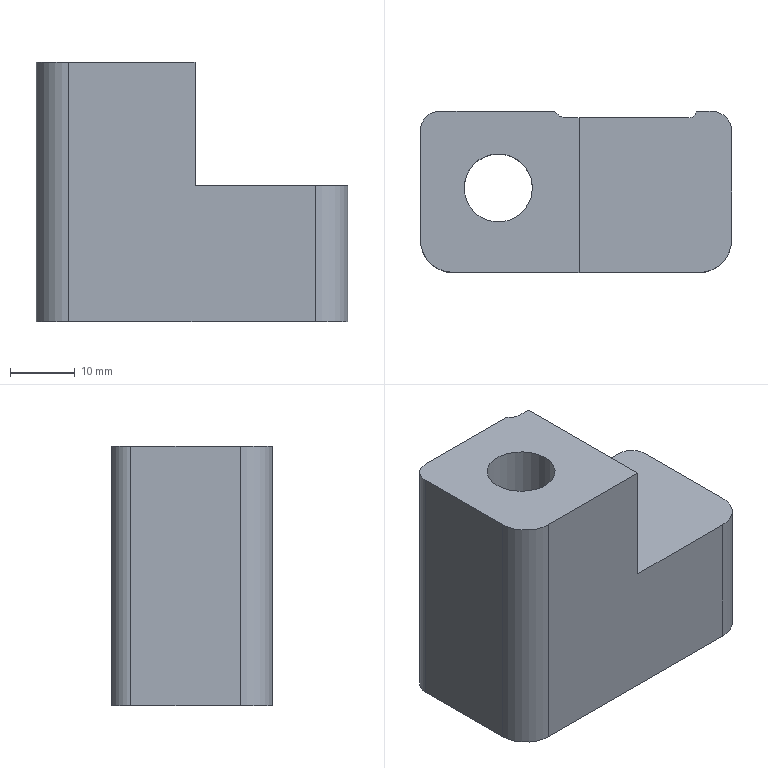Part | NX | features PS-11 2 | 1 solid | 19 faces | box 47.924 x 24.8 x 40 mm | volume 29874 mm3 | plane 11 | cylinder 8 | commonest cylinder face diameters 6 x2 10 x2 2.4 x1 4.4 x1 10.5 x1 18 x1
STEP:
#1=CARTESIAN_POINT('',(2543.009,-914.397,881.716));
#2=VERTEX_POINT('',#1);
#3=CARTESIAN_POINT('',(2543.009,-938.197,881.716));
#4=VERTEX_POINT('',#3);
#5=CARTESIAN_POINT('',(2543.009,-857.123,881.716));
#6=DIRECTION('',(0.,-1.,0.));
#7=VECTOR('',#6,1000.);
#8=LINE('',#5,#7);
#9=EDGE_CURVE('',#2,#4,#8,.T.);
#10=ORIENTED_EDGE('',*,*,#9,.F.);
#11=CARTESIAN_POINT('',(2543.009,-914.397,900.716));
#12=VERTEX_POINT('',#11);
#13=CARTESIAN_POINT('',(2543.009,-914.397,940.716));
#14=DIRECTION('',(0.,0.,-1.));
#15=VECTOR('',#14,1000.);
#16=LINE('',#13,#15);
#17=EDGE_CURVE('',#12,#2,#16,.T.);
#18=ORIENTED_EDGE('',*,*,#17,.F.);
#19=CARTESIAN_POINT('',(2543.009,-938.197,900.716));
#20=VERTEX_POINT('',#19);
#21=CARTESIAN_POINT('',(2543.009,-857.123,900.716));
#22=DIRECTION('',(0.,-1.,0.));
#23=VECTOR('',#22,1000.);
#24=LINE('',#21,#23);
#25=EDGE_CURVE('',#20,#12,#24,.F.);
#26=ORIENTED_EDGE('',*,*,#25,.F.);
#27=CARTESIAN_POINT('',(2543.009,-938.197,853.217));
#28=DIRECTION('',(0.,0.,-1.));
#29=VECTOR('',#28,1000.);
#30=LINE('',#27,#29);
#31=EDGE_CURVE('',#4,#20,#30,.F.);
#32=ORIENTED_EDGE('',*,*,#31,.F.);
#33=EDGE_LOOP('',(#10,#18,#26,#32));
#34=FACE_BOUND('',#33,.T.);
#35=CARTESIAN_POINT('',(2543.009,-923.947,911.056));
#36=DIRECTION('',(-1.,0.,0.));
#37=DIRECTION('',(0.,0.,1.));
#38=AXIS2_PLACEMENT_3D('',#35,#36,#37);
#39=PLANE('',#38);
#40=ADVANCED_FACE('',(#34),#39,.F.);
#41=CARTESIAN_POINT('',(2559.923,-914.397,860.716));
#42=VERTEX_POINT('',#41);
#43=CARTESIAN_POINT('',(2541.096,-914.397,860.716));
#44=VERTEX_POINT('',#43);
#45=CARTESIAN_POINT('',(2585.094,-914.397,860.716));
#46=DIRECTION('',(-1.,0.,0.));
#47=VECTOR('',#46,1000.);
#48=LINE('',#45,#47);
#49=EDGE_CURVE('',#42,#44,#48,.T.);
#50=ORIENTED_EDGE('',*,*,#49,.F.);
#51=CARTESIAN_POINT('',(2561.106,-913.397,860.716));
#52=VERTEX_POINT('',#51);
#53=CARTESIAN_POINT('',(2559.923,-913.197,860.716));
#54=DIRECTION('',(0.,0.,-1.));
#55=DIRECTION('',(-1.,0.,0.));
#56=AXIS2_PLACEMENT_3D('',#53,#54,#55);
#57=CIRCLE('',#56,1.2);
#58=EDGE_CURVE('',#52,#42,#57,.T.);
#59=ORIENTED_EDGE('',*,*,#58,.F.);
#60=CARTESIAN_POINT('',(2563.509,-913.397,860.716));
#61=VERTEX_POINT('',#60);
#62=CARTESIAN_POINT('',(2585.094,-913.397,860.716));
#63=DIRECTION('',(1.,0.,0.));
#64=VECTOR('',#63,1000.);
#65=LINE('',#62,#64);
#66=EDGE_CURVE('',#52,#61,#65,.T.);
#67=ORIENTED_EDGE('',*,*,#66,.T.);
#68=CARTESIAN_POINT('',(2566.509,-916.397,860.716));
#69=VERTEX_POINT('',#68);
#70=CARTESIAN_POINT('',(2563.509,-916.397,860.716));
#71=DIRECTION('',(0.,0.,-1.));
#72=DIRECTION('',(-1.,0.,0.));
#73=AXIS2_PLACEMENT_3D('',#70,#71,#72);
#74=CIRCLE('',#73,3.);
#75=EDGE_CURVE('',#61,#69,#74,.T.);
#76=ORIENTED_EDGE('',*,*,#75,.T.);
#77=CARTESIAN_POINT('',(2566.509,-933.197,860.716));
#78=VERTEX_POINT('',#77);
#79=CARTESIAN_POINT('',(2566.509,-906.16,860.716));
#80=DIRECTION('',(0.,1.,0.));
#81=VECTOR('',#80,1000.);
#82=LINE('',#79,#81);
#83=EDGE_CURVE('',#78,#69,#82,.T.);
#84=ORIENTED_EDGE('',*,*,#83,.F.);
#85=CARTESIAN_POINT('',(2561.509,-938.197,860.716));
#86=VERTEX_POINT('',#85);
#87=CARTESIAN_POINT('',(2561.509,-933.197,860.716));
#88=DIRECTION('',(0.,0.,1.));
#89=DIRECTION('',(-1.,0.,0.));
#90=AXIS2_PLACEMENT_3D('',#87,#88,#89);
#91=CIRCLE('',#90,5.);
#92=EDGE_CURVE('',#86,#78,#91,.T.);
#93=ORIENTED_EDGE('',*,*,#92,.F.);
#94=CARTESIAN_POINT('',(2523.585,-938.197,860.716));
#95=VERTEX_POINT('',#94);
#96=CARTESIAN_POINT('',(2524.047,-938.197,860.716));
#97=DIRECTION('',(-1.,0.,0.));
#98=VECTOR('',#97,1000.);
#99=LINE('',#96,#98);
#100=EDGE_CURVE('',#86,#95,#99,.T.);
#101=ORIENTED_EDGE('',*,*,#100,.T.);
#102=CARTESIAN_POINT('',(2518.585,-933.197,860.716));
#103=VERTEX_POINT('',#102);
#104=CARTESIAN_POINT('',(2523.585,-933.197,860.716));
#105=DIRECTION('',(0.,0.,1.));
#106=DIRECTION('',(-1.,0.,0.));
#107=AXIS2_PLACEMENT_3D('',#104,#105,#106);
#108=CIRCLE('',#107,5.);
#109=EDGE_CURVE('',#103,#95,#108,.T.);
#110=ORIENTED_EDGE('',*,*,#109,.F.);
#111=CARTESIAN_POINT('',(2518.585,-916.397,860.716));
#112=VERTEX_POINT('',#111);
#113=CARTESIAN_POINT('',(2518.585,-924.697,860.716));
#114=DIRECTION('',(0.,1.,0.));
#115=VECTOR('',#114,1000.);
#116=LINE('',#113,#115);
#117=EDGE_CURVE('',#103,#112,#116,.T.);
#118=ORIENTED_EDGE('',*,*,#117,.T.);
#119=CARTESIAN_POINT('',(2521.585,-913.397,860.716));
#120=VERTEX_POINT('',#119);
#121=CARTESIAN_POINT('',(2521.585,-916.397,860.716));
#122=DIRECTION('',(0.,0.,-1.));
#123=DIRECTION('',(-1.,0.,0.));
#124=AXIS2_PLACEMENT_3D('',#121,#122,#123);
#125=CIRCLE('',#124,3.);
#126=EDGE_CURVE('',#112,#120,#125,.T.);
#127=ORIENTED_EDGE('',*,*,#126,.T.);
#128=CARTESIAN_POINT('',(2539.252,-913.397,860.716));
#129=VERTEX_POINT('',#128);
#130=CARTESIAN_POINT('',(2585.094,-913.397,860.716));
#131=DIRECTION('',(1.,0.,0.));
#132=VECTOR('',#131,1000.);
#133=LINE('',#130,#132);
#134=EDGE_CURVE('',#120,#129,#133,.T.);
#135=ORIENTED_EDGE('',*,*,#134,.T.);
#136=CARTESIAN_POINT('',(2541.096,-912.197,860.716));
#137=DIRECTION('',(0.,0.,-1.));
#138=DIRECTION('',(-1.,0.,0.));
#139=AXIS2_PLACEMENT_3D('',#136,#137,#138);
#140=CIRCLE('',#139,2.2);
#141=EDGE_CURVE('',#129,#44,#140,.F.);
#142=ORIENTED_EDGE('',*,*,#141,.T.);
#143=EDGE_LOOP('',(#50,#59,#67,#76,#84,#93,#101,#110,#118,#127,#135,#142));
#144=FACE_BOUND('',#143,.T.);
#145=CARTESIAN_POINT('',(2521.585,-925.197,860.716));
#146=VERTEX_POINT('',#145);
#147=CARTESIAN_POINT('',(2530.585,-925.197,860.716));
#148=DIRECTION('',(0.,0.,1.));
#149=DIRECTION('',(-1.,0.,0.));
#150=AXIS2_PLACEMENT_3D('',#147,#148,#149);
#151=CIRCLE('',#150,9.);
#152=EDGE_CURVE('',#146,#146,#151,.T.);
#153=ORIENTED_EDGE('',*,*,#152,.T.);
#154=EDGE_LOOP('',(#153));
#155=FACE_BOUND('',#154,.T.);
#156=CARTESIAN_POINT('',(2585.094,-857.123,860.716));
#157=DIRECTION('',(0.,0.,-1.));
#158=DIRECTION('',(-1.,0.,0.));
#159=AXIS2_PLACEMENT_3D('',#156,#157,#158);
#160=PLANE('',#159);
#161=ADVANCED_FACE('',(#144,#155),#160,.T.);
#162=ORIENTED_EDGE('',*,*,#25,.T.);
#163=CARTESIAN_POINT('',(2541.096,-914.397,900.716));
#164=VERTEX_POINT('',#163);
#165=CARTESIAN_POINT('',(2585.094,-914.397,900.716));
#166=DIRECTION('',(1.,0.,0.));
#167=VECTOR('',#166,1000.);
#168=LINE('',#165,#167);
#169=EDGE_CURVE('',#164,#12,#168,.T.);
#170=ORIENTED_EDGE('',*,*,#169,.F.);
#171=CARTESIAN_POINT('',(2539.252,-913.397,900.716));
#172=VERTEX_POINT('',#171);
#173=CARTESIAN_POINT('',(2541.096,-912.197,900.716));
#174=DIRECTION('',(0.,0.,1.));
#175=DIRECTION('',(1.,0.,0.));
#176=AXIS2_PLACEMENT_3D('',#173,#174,#175);
#177=CIRCLE('',#176,2.2);
#178=EDGE_CURVE('',#164,#172,#177,.F.);
#179=ORIENTED_EDGE('',*,*,#178,.T.);
#180=CARTESIAN_POINT('',(2521.585,-913.397,900.716));
#181=VERTEX_POINT('',#180);
#182=CARTESIAN_POINT('',(2585.094,-913.397,900.716));
#183=DIRECTION('',(-1.,0.,0.));
#184=VECTOR('',#183,1000.);
#185=LINE('',#182,#184);
#186=EDGE_CURVE('',#172,#181,#185,.T.);
#187=ORIENTED_EDGE('',*,*,#186,.T.);
#188=CARTESIAN_POINT('',(2518.585,-916.397,900.716));
#189=VERTEX_POINT('',#188);
#190=CARTESIAN_POINT('',(2521.585,-916.397,900.716));
#191=DIRECTION('',(0.,0.,1.));
#192=DIRECTION('',(1.,0.,0.));
#193=AXIS2_PLACEMENT_3D('',#190,#191,#192);
#194=CIRCLE('',#193,3.);
#195=EDGE_CURVE('',#181,#189,#194,.T.);
#196=ORIENTED_EDGE('',*,*,#195,.T.);
#197=CARTESIAN_POINT('',(2518.585,-933.197,900.716));
#198=VERTEX_POINT('',#197);
#199=CARTESIAN_POINT('',(2518.585,-924.697,900.716));
#200=DIRECTION('',(0.,1.,0.));
#201=VECTOR('',#200,1000.);
#202=LINE('',#199,#201);
#203=EDGE_CURVE('',#198,#189,#202,.T.);
#204=ORIENTED_EDGE('',*,*,#203,.F.);
#205=CARTESIAN_POINT('',(2523.585,-938.197,900.716));
#206=VERTEX_POINT('',#205);
#207=CARTESIAN_POINT('',(2523.585,-933.197,900.716));
#208=DIRECTION('',(0.,0.,1.));
#209=DIRECTION('',(1.,0.,0.));
#210=AXIS2_PLACEMENT_3D('',#207,#208,#209);
#211=CIRCLE('',#210,5.);
#212=EDGE_CURVE('',#206,#198,#211,.F.);
#213=ORIENTED_EDGE('',*,*,#212,.F.);
#214=CARTESIAN_POINT('',(2524.047,-938.197,900.716));
#215=DIRECTION('',(-1.,0.,0.));
#216=VECTOR('',#215,1000.);
#217=LINE('',#214,#216);
#218=EDGE_CURVE('',#20,#206,#217,.T.);
#219=ORIENTED_EDGE('',*,*,#218,.F.);
#220=EDGE_LOOP('',(#162,#170,#179,#187,#196,#204,#213,#219));
#221=FACE_BOUND('',#220,.T.);
#222=CARTESIAN_POINT('',(2535.835,-925.197,900.716));
#223=VERTEX_POINT('',#222);
#224=CARTESIAN_POINT('',(2530.585,-925.197,900.716));
#225=DIRECTION('',(0.,0.,1.));
#226=DIRECTION('',(1.,0.,0.));
#227=AXIS2_PLACEMENT_3D('',#224,#225,#226);
#228=CIRCLE('',#227,5.25);
#229=EDGE_CURVE('',#223,#223,#228,.F.);
#230=ORIENTED_EDGE('',*,*,#229,.T.);
#231=EDGE_LOOP('',(#230));
#232=FACE_BOUND('',#231,.T.);
#233=CARTESIAN_POINT('',(2585.094,-857.123,900.716));
#234=DIRECTION('',(0.,0.,1.));
#235=DIRECTION('',(1.,0.,0.));
#236=AXIS2_PLACEMENT_3D('',#233,#234,#235);
#237=PLANE('',#236);
#238=ADVANCED_FACE('',(#221,#232),#237,.T.);
#239=ORIENTED_EDGE('',*,*,#141,.F.);
#240=CARTESIAN_POINT('',(2539.252,-913.397,889.83));
#241=DIRECTION('',(0.,0.,-1.));
#242=VECTOR('',#241,1000.);
#243=LINE('',#240,#242);
#244=EDGE_CURVE('',#129,#172,#243,.F.);
#245=ORIENTED_EDGE('',*,*,#244,.T.);
#246=ORIENTED_EDGE('',*,*,#178,.F.);
#247=CARTESIAN_POINT('',(2541.096,-914.397,940.716));
#248=DIRECTION('',(0.,0.,-1.));
#249=VECTOR('',#248,1000.);
#250=LINE('',#247,#249);
#251=EDGE_CURVE('',#44,#164,#250,.F.);
#252=ORIENTED_EDGE('',*,*,#251,.F.);
#253=EDGE_LOOP('',(#239,#245,#246,#252));
#254=FACE_BOUND('',#253,.T.);
#255=CARTESIAN_POINT('',(2541.096,-912.197,889.83));
#256=DIRECTION('',(0.,0.,-1.));
#257=DIRECTION('',(-1.,0.,0.));
#258=AXIS2_PLACEMENT_3D('',#255,#256,#257);
#259=CYLINDRICAL_SURFACE('',#258,2.2);
#260=ADVANCED_FACE('',(#254),#259,.F.);
#261=ORIENTED_EDGE('',*,*,#100,.F.);
#262=CARTESIAN_POINT('',(2561.509,-938.197,881.716));
#263=VERTEX_POINT('',#262);
#264=CARTESIAN_POINT('',(2561.509,-938.197,853.217));
#265=DIRECTION('',(0.,0.,1.));
#266=VECTOR('',#265,1000.);
#267=LINE('',#264,#266);
#268=EDGE_CURVE('',#263,#86,#267,.F.);
#269=ORIENTED_EDGE('',*,*,#268,.F.);
#270=CARTESIAN_POINT('',(2524.047,-938.197,881.716));
#271=DIRECTION('',(-1.,0.,0.));
#272=VECTOR('',#271,1000.);
#273=LINE('',#270,#272);
#274=EDGE_CURVE('',#263,#4,#273,.T.);
#275=ORIENTED_EDGE('',*,*,#274,.T.);
#276=ORIENTED_EDGE('',*,*,#31,.T.);
#277=ORIENTED_EDGE('',*,*,#218,.T.);
#278=CARTESIAN_POINT('',(2523.585,-938.197,853.217));
#279=DIRECTION('',(0.,0.,1.));
#280=VECTOR('',#279,1000.);
#281=LINE('',#278,#280);
#282=EDGE_CURVE('',#95,#206,#281,.T.);
#283=ORIENTED_EDGE('',*,*,#282,.F.);
#284=EDGE_LOOP('',(#261,#269,#275,#276,#277,#283));
#285=FACE_BOUND('',#284,.T.);
#286=CARTESIAN_POINT('',(2524.047,-938.197,853.217));
#287=DIRECTION('',(0.,-1.,0.));
#288=DIRECTION('',(0.,0.,1.));
#289=AXIS2_PLACEMENT_3D('',#286,#287,#288);
#290=PLANE('',#289);
#291=ADVANCED_FACE('',(#285),#290,.T.);
#292=ORIENTED_EDGE('',*,*,#203,.T.);
#293=CARTESIAN_POINT('',(2518.585,-916.397,875.716));
#294=DIRECTION('',(0.,0.,-1.));
#295=VECTOR('',#294,1000.);
#296=LINE('',#293,#295);
#297=EDGE_CURVE('',#189,#112,#296,.T.);
#298=ORIENTED_EDGE('',*,*,#297,.T.);
#299=ORIENTED_EDGE('',*,*,#117,.F.);
#300=CARTESIAN_POINT('',(2518.585,-933.197,875.716));
#301=DIRECTION('',(0.,0.,1.));
#302=VECTOR('',#301,1000.);
#303=LINE('',#300,#302);
#304=EDGE_CURVE('',#198,#103,#303,.F.);
#305=ORIENTED_EDGE('',*,*,#304,.F.);
#306=EDGE_LOOP('',(#292,#298,#299,#305));
#307=FACE_BOUND('',#306,.T.);
#308=CARTESIAN_POINT('',(2518.585,-924.697,875.716));
#309=DIRECTION('',(-1.,0.,0.));
#310=DIRECTION('',(0.,0.,1.));
#311=AXIS2_PLACEMENT_3D('',#308,#309,#310);
#312=PLANE('',#311);
#313=ADVANCED_FACE('',(#307),#312,.T.);
#314=ORIENTED_EDGE('',*,*,#109,.T.);
#315=ORIENTED_EDGE('',*,*,#282,.T.);
#316=ORIENTED_EDGE('',*,*,#212,.T.);
#317=ORIENTED_EDGE('',*,*,#304,.T.);
#318=EDGE_LOOP('',(#314,#315,#316,#317));
#319=FACE_BOUND('',#318,.T.);
#320=CARTESIAN_POINT('',(2523.585,-933.197,853.217));
#321=DIRECTION('',(0.,0.,1.));
#322=DIRECTION('',(1.,0.,0.));
#323=AXIS2_PLACEMENT_3D('',#320,#321,#322);
#324=CYLINDRICAL_SURFACE('',#323,5.);
#325=ADVANCED_FACE('',(#319),#324,.T.);
#326=ORIENTED_EDGE('',*,*,#229,.F.);
#327=EDGE_LOOP('',(#326));
#328=FACE_BOUND('',#327,.T.);
#329=CARTESIAN_POINT('',(2525.335,-925.197,873.716));
#330=VERTEX_POINT('',#329);
#331=CARTESIAN_POINT('',(2530.585,-925.197,873.716));
#332=DIRECTION('',(0.,0.,1.));
#333=DIRECTION('',(-1.,0.,0.));
#334=AXIS2_PLACEMENT_3D('',#331,#332,#333);
#335=CIRCLE('',#334,5.25);
#336=EDGE_CURVE('',#330,#330,#335,.T.);
#337=ORIENTED_EDGE('',*,*,#336,.F.);
#338=EDGE_LOOP('',(#337));
#339=FACE_BOUND('',#338,.T.);
#340=CARTESIAN_POINT('',(2530.585,-925.197,891.716));
#341=DIRECTION('',(0.,0.,-1.));
#342=DIRECTION('',(-1.,0.,0.));
#343=AXIS2_PLACEMENT_3D('',#340,#341,#342);
#344=CYLINDRICAL_SURFACE('',#343,5.25);
#345=ADVANCED_FACE('',(#328,#339),#344,.F.);
#346=ORIENTED_EDGE('',*,*,#152,.F.);
#347=EDGE_LOOP('',(#346));
#348=FACE_BOUND('',#347,.T.);
#349=CARTESIAN_POINT('',(2539.585,-925.197,873.716));
#350=VERTEX_POINT('',#349);
#351=CARTESIAN_POINT('',(2530.585,-925.197,873.716));
#352=DIRECTION('',(0.,0.,1.));
#353=DIRECTION('',(1.,0.,0.));
#354=AXIS2_PLACEMENT_3D('',#351,#352,#353);
#355=CIRCLE('',#354,9.);
#356=EDGE_CURVE('',#350,#350,#355,.F.);
#357=ORIENTED_EDGE('',*,*,#356,.F.);
#358=EDGE_LOOP('',(#357));
#359=FACE_BOUND('',#358,.T.);
#360=CARTESIAN_POINT('',(2530.585,-925.197,873.716));
#361=DIRECTION('',(0.,0.,-1.));
#362=DIRECTION('',(-1.,0.,0.));
#363=AXIS2_PLACEMENT_3D('',#360,#361,#362);
#364=CYLINDRICAL_SURFACE('',#363,9.);
#365=ADVANCED_FACE('',(#348,#359),#364,.F.);
#366=ORIENTED_EDGE('',*,*,#336,.T.);
#367=EDGE_LOOP('',(#366));
#368=FACE_BOUND('',#367,.T.);
#369=ORIENTED_EDGE('',*,*,#356,.T.);
#370=EDGE_LOOP('',(#369));
#371=FACE_BOUND('',#370,.T.);
#372=CARTESIAN_POINT('',(2530.585,-925.197,873.716));
#373=DIRECTION('',(0.,0.,-1.));
#374=DIRECTION('',(-1.,0.,0.));
#375=AXIS2_PLACEMENT_3D('',#372,#373,#374);
#376=PLANE('',#375);
#377=ADVANCED_FACE('',(#368,#371),#376,.T.);
#378=ORIENTED_EDGE('',*,*,#169,.T.);
#379=ORIENTED_EDGE('',*,*,#17,.T.);
#380=CARTESIAN_POINT('',(2559.923,-914.397,881.716));
#381=VERTEX_POINT('',#380);
#382=CARTESIAN_POINT('',(2585.094,-914.397,881.716));
#383=DIRECTION('',(1.,0.,0.));
#384=VECTOR('',#383,1000.);
#385=LINE('',#382,#384);
#386=EDGE_CURVE('',#2,#381,#385,.T.);
#387=ORIENTED_EDGE('',*,*,#386,.T.);
#388=CARTESIAN_POINT('',(2559.923,-914.397,940.716));
#389=DIRECTION('',(0.,0.,-1.));
#390=VECTOR('',#389,1000.);
#391=LINE('',#388,#390);
#392=EDGE_CURVE('',#42,#381,#391,.F.);
#393=ORIENTED_EDGE('',*,*,#392,.F.);
#394=ORIENTED_EDGE('',*,*,#49,.T.);
#395=ORIENTED_EDGE('',*,*,#251,.T.);
#396=EDGE_LOOP('',(#378,#379,#387,#393,#394,#395));
#397=FACE_BOUND('',#396,.T.);
#398=CARTESIAN_POINT('',(2656.665,-914.397,940.716));
#399=DIRECTION('',(0.,-1.,0.));
#400=DIRECTION('',(0.,0.,-1.));
#401=AXIS2_PLACEMENT_3D('',#398,#399,#400);
#402=PLANE('',#401);
#403=ADVANCED_FACE('',(#397),#402,.F.);
#404=ORIENTED_EDGE('',*,*,#134,.F.);
#405=CARTESIAN_POINT('',(2521.585,-913.397,875.716));
#406=DIRECTION('',(0.,0.,-1.));
#407=VECTOR('',#406,1000.);
#408=LINE('',#405,#407);
#409=EDGE_CURVE('',#120,#181,#408,.F.);
#410=ORIENTED_EDGE('',*,*,#409,.T.);
#411=ORIENTED_EDGE('',*,*,#186,.F.);
#412=ORIENTED_EDGE('',*,*,#244,.F.);
#413=EDGE_LOOP('',(#404,#410,#411,#412));
#414=FACE_BOUND('',#413,.T.);
#415=CARTESIAN_POINT('',(2550.509,-913.397,875.716));
#416=DIRECTION('',(0.,1.,0.));
#417=DIRECTION('',(0.,0.,1.));
#418=AXIS2_PLACEMENT_3D('',#415,#416,#417);
#419=PLANE('',#418);
#420=ADVANCED_FACE('',(#414),#419,.T.);
#421=ORIENTED_EDGE('',*,*,#195,.F.);
#422=ORIENTED_EDGE('',*,*,#409,.F.);
#423=ORIENTED_EDGE('',*,*,#126,.F.);
#424=ORIENTED_EDGE('',*,*,#297,.F.);
#425=EDGE_LOOP('',(#421,#422,#423,#424));
#426=FACE_BOUND('',#425,.T.);
#427=CARTESIAN_POINT('',(2521.585,-916.397,875.716));
#428=DIRECTION('',(0.,0.,-1.));
#429=DIRECTION('',(-1.,0.,0.));
#430=AXIS2_PLACEMENT_3D('',#427,#428,#429);
#431=CYLINDRICAL_SURFACE('',#430,3.);
#432=ADVANCED_FACE('',(#426),#431,.T.);
#433=CARTESIAN_POINT('',(2563.509,-913.397,881.716));
#434=VERTEX_POINT('',#433);
#435=CARTESIAN_POINT('',(2561.106,-913.397,881.716));
#436=VERTEX_POINT('',#435);
#437=CARTESIAN_POINT('',(2585.094,-913.397,881.716));
#438=DIRECTION('',(-1.,0.,0.));
#439=VECTOR('',#438,1000.);
#440=LINE('',#437,#439);
#441=EDGE_CURVE('',#434,#436,#440,.T.);
#442=ORIENTED_EDGE('',*,*,#441,.F.);
#443=CARTESIAN_POINT('',(2563.509,-913.397,875.716));
#444=DIRECTION('',(0.,0.,1.));
#445=VECTOR('',#444,1000.);
#446=LINE('',#443,#445);
#447=EDGE_CURVE('',#434,#61,#446,.F.);
#448=ORIENTED_EDGE('',*,*,#447,.T.);
#449=ORIENTED_EDGE('',*,*,#66,.F.);
#450=CARTESIAN_POINT('',(2561.106,-913.397,940.716));
#451=DIRECTION('',(0.,0.,-1.));
#452=VECTOR('',#451,1000.);
#453=LINE('',#450,#452);
#454=EDGE_CURVE('',#52,#436,#453,.F.);
#455=ORIENTED_EDGE('',*,*,#454,.T.);
#456=EDGE_LOOP('',(#442,#448,#449,#455));
#457=FACE_BOUND('',#456,.T.);
#458=CARTESIAN_POINT('',(2550.509,-913.397,875.716));
#459=DIRECTION('',(0.,1.,0.));
#460=DIRECTION('',(0.,0.,1.));
#461=AXIS2_PLACEMENT_3D('',#458,#459,#460);
#462=PLANE('',#461);
#463=ADVANCED_FACE('',(#457),#462,.T.);
#464=ORIENTED_EDGE('',*,*,#75,.F.);
#465=ORIENTED_EDGE('',*,*,#447,.F.);
#466=CARTESIAN_POINT('',(2566.509,-916.397,881.716));
#467=VERTEX_POINT('',#466);
#468=CARTESIAN_POINT('',(2563.509,-916.397,881.716));
#469=DIRECTION('',(0.,0.,1.));
#470=DIRECTION('',(1.,0.,0.));
#471=AXIS2_PLACEMENT_3D('',#468,#469,#470);
#472=CIRCLE('',#471,3.);
#473=EDGE_CURVE('',#467,#434,#472,.T.);
#474=ORIENTED_EDGE('',*,*,#473,.F.);
#475=CARTESIAN_POINT('',(2566.509,-916.397,853.217));
#476=DIRECTION('',(0.,0.,1.));
#477=VECTOR('',#476,1000.);
#478=LINE('',#475,#477);
#479=EDGE_CURVE('',#69,#467,#478,.T.);
#480=ORIENTED_EDGE('',*,*,#479,.F.);
#481=EDGE_LOOP('',(#464,#465,#474,#480));
#482=FACE_BOUND('',#481,.T.);
#483=CARTESIAN_POINT('',(2563.509,-916.397,853.217));
#484=DIRECTION('',(0.,0.,1.));
#485=DIRECTION('',(1.,0.,0.));
#486=AXIS2_PLACEMENT_3D('',#483,#484,#485);
#487=CYLINDRICAL_SURFACE('',#486,3.);
#488=ADVANCED_FACE('',(#482),#487,.T.);
#489=ORIENTED_EDGE('',*,*,#83,.T.);
#490=ORIENTED_EDGE('',*,*,#479,.T.);
#491=CARTESIAN_POINT('',(2566.509,-933.197,881.716));
#492=VERTEX_POINT('',#491);
#493=CARTESIAN_POINT('',(2566.509,-906.16,881.716));
#494=DIRECTION('',(0.,-1.,0.));
#495=VECTOR('',#494,1000.);
#496=LINE('',#493,#495);
#497=EDGE_CURVE('',#467,#492,#496,.T.);
#498=ORIENTED_EDGE('',*,*,#497,.T.);
#499=CARTESIAN_POINT('',(2566.509,-933.197,853.217));
#500=DIRECTION('',(0.,0.,1.));
#501=VECTOR('',#500,1000.);
#502=LINE('',#499,#501);
#503=EDGE_CURVE('',#78,#492,#502,.T.);
#504=ORIENTED_EDGE('',*,*,#503,.F.);
#505=EDGE_LOOP('',(#489,#490,#498,#504));
#506=FACE_BOUND('',#505,.T.);
#507=CARTESIAN_POINT('',(2566.509,-906.16,853.217));
#508=DIRECTION('',(1.,0.,0.));
#509=DIRECTION('',(0.,0.,-1.));
#510=AXIS2_PLACEMENT_3D('',#507,#508,#509);
#511=PLANE('',#510);
#512=ADVANCED_FACE('',(#506),#511,.T.);
#513=ORIENTED_EDGE('',*,*,#92,.T.);
#514=ORIENTED_EDGE('',*,*,#503,.T.);
#515=CARTESIAN_POINT('',(2561.509,-933.197,881.716));
#516=DIRECTION('',(0.,0.,1.));
#517=DIRECTION('',(1.,0.,0.));
#518=AXIS2_PLACEMENT_3D('',#515,#516,#517);
#519=CIRCLE('',#518,5.);
#520=EDGE_CURVE('',#492,#263,#519,.F.);
#521=ORIENTED_EDGE('',*,*,#520,.T.);
#522=ORIENTED_EDGE('',*,*,#268,.T.);
#523=EDGE_LOOP('',(#513,#514,#521,#522));
#524=FACE_BOUND('',#523,.T.);
#525=CARTESIAN_POINT('',(2561.509,-933.197,853.217));
#526=DIRECTION('',(0.,0.,1.));
#527=DIRECTION('',(1.,0.,0.));
#528=AXIS2_PLACEMENT_3D('',#525,#526,#527);
#529=CYLINDRICAL_SURFACE('',#528,5.);
#530=ADVANCED_FACE('',(#524),#529,.T.);
#531=ORIENTED_EDGE('',*,*,#454,.F.);
#532=ORIENTED_EDGE('',*,*,#58,.T.);
#533=ORIENTED_EDGE('',*,*,#392,.T.);
#534=CARTESIAN_POINT('',(2559.923,-913.197,881.716));
#535=DIRECTION('',(0.,0.,1.));
#536=DIRECTION('',(1.,0.,0.));
#537=AXIS2_PLACEMENT_3D('',#534,#535,#536);
#538=CIRCLE('',#537,1.2);
#539=EDGE_CURVE('',#381,#436,#538,.T.);
#540=ORIENTED_EDGE('',*,*,#539,.T.);
#541=EDGE_LOOP('',(#531,#532,#533,#540));
#542=FACE_BOUND('',#541,.T.);
#543=CARTESIAN_POINT('',(2559.923,-913.197,940.716));
#544=DIRECTION('',(0.,0.,-1.));
#545=DIRECTION('',(-1.,0.,0.));
#546=AXIS2_PLACEMENT_3D('',#543,#544,#545);
#547=CYLINDRICAL_SURFACE('',#546,1.2);
#548=ADVANCED_FACE('',(#542),#547,.F.);
#549=ORIENTED_EDGE('',*,*,#386,.F.);
#550=ORIENTED_EDGE('',*,*,#9,.T.);
#551=ORIENTED_EDGE('',*,*,#274,.F.);
#552=ORIENTED_EDGE('',*,*,#520,.F.);
#553=ORIENTED_EDGE('',*,*,#497,.F.);
#554=ORIENTED_EDGE('',*,*,#473,.T.);
#555=ORIENTED_EDGE('',*,*,#441,.T.);
#556=ORIENTED_EDGE('',*,*,#539,.F.);
#557=EDGE_LOOP('',(#549,#550,#551,#552,#553,#554,#555,#556));
#558=FACE_BOUND('',#557,.T.);
#559=CARTESIAN_POINT('',(2585.094,-857.123,881.716));
#560=DIRECTION('',(0.,0.,1.));
#561=DIRECTION('',(1.,0.,0.));
#562=AXIS2_PLACEMENT_3D('',#559,#560,#561);
#563=PLANE('',#562);
#564=ADVANCED_FACE('',(#558),#563,.T.);
#565=CLOSED_SHELL('',(#40,#161,#238,#260,#291,#313,#325,#345,#365,#377,#403,#420,#432,#463,#488,#512,#530,#548,#564));
#566=MANIFOLD_SOLID_BREP('',#565);
#567=(LENGTH_UNIT()NAMED_UNIT(*)SI_UNIT(.MILLI.,.METRE.));
#568=UNCERTAINTY_MEASURE_WITH_UNIT(LENGTH_MEASURE(0.00001),#567,'','');
#569=(NAMED_UNIT(*)PLANE_ANGLE_UNIT()SI_UNIT($,.RADIAN.));
#570=(NAMED_UNIT(*)SI_UNIT($,.STERADIAN.)SOLID_ANGLE_UNIT());
#571=(GEOMETRIC_REPRESENTATION_CONTEXT(3)GLOBAL_UNCERTAINTY_ASSIGNED_CONTEXT((#568))GLOBAL_UNIT_ASSIGNED_CONTEXT((#567,#569,#570))REPRESENTATION_CONTEXT('',''));
#572=ADVANCED_BREP_SHAPE_REPRESENTATION('',(#566),#571);